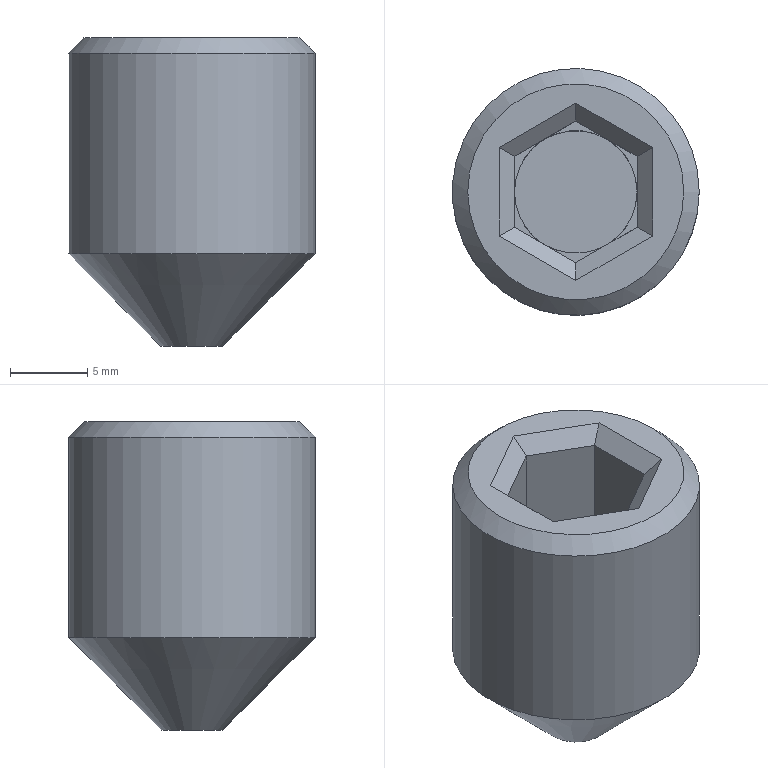Part | NX | features solid 2 | 1 solid | 25 faces | box 16 x 16 x 20 mm | volume 2801 mm3 | plane 21 | cylinder 2 | cone 2 | commonest cylinder face diameters 7.951 x1 16 x1
STEP:
#1=CARTESIAN_POINT('',(-112.,-5.,-5.));
#2=VERTEX_POINT('',#1);
#3=CARTESIAN_POINT('',(-120.,-5.,-5.));
#4=DIRECTION('',(0.,0.,1.));
#5=DIRECTION('',(1.,0.,0.));
#6=AXIS2_PLACEMENT_3D('',#3,#4,#5);
#7=CIRCLE('',#6,8.);
#8=EDGE_CURVE('',#2,#2,#7,.F.);
#9=ORIENTED_EDGE('',*,*,#8,.T.);
#10=EDGE_LOOP('',(#9));
#11=FACE_BOUND('',#10,.T.);
#12=CARTESIAN_POINT('',(-112.,-5.,-18.));
#13=VERTEX_POINT('',#12);
#14=CARTESIAN_POINT('',(-120.,-5.,-18.));
#15=DIRECTION('',(0.,0.,1.));
#16=DIRECTION('',(1.,0.,0.));
#17=AXIS2_PLACEMENT_3D('',#14,#15,#16);
#18=CIRCLE('',#17,8.);
#19=EDGE_CURVE('',#13,#13,#18,.F.);
#20=ORIENTED_EDGE('',*,*,#19,.F.);
#21=EDGE_LOOP('',(#20));
#22=FACE_BOUND('',#21,.T.);
#23=CARTESIAN_POINT('',(-120.,-5.,36.));
#24=DIRECTION('',(0.,0.,-1.));
#25=DIRECTION('',(-1.,0.,0.));
#26=AXIS2_PLACEMENT_3D('',#23,#24,#25);
#27=CYLINDRICAL_SURFACE('',#26,8.);
#28=ADVANCED_FACE('',(#11,#22),#27,.T.);
#29=CARTESIAN_POINT('',(-123.976,-5.,-11.));
#30=VERTEX_POINT('',#29);
#31=CARTESIAN_POINT('',(-121.988,-8.443,-11.));
#32=VERTEX_POINT('',#31);
#33=CARTESIAN_POINT('',(-120.,-5.,-11.));
#34=DIRECTION('',(0.,0.,-1.));
#35=DIRECTION('',(-1.,0.,0.));
#36=AXIS2_PLACEMENT_3D('',#33,#34,#35);
#37=CIRCLE('',#36,3.976);
#38=EDGE_CURVE('',#30,#32,#37,.F.);
#39=ORIENTED_EDGE('',*,*,#38,.F.);
#40=CARTESIAN_POINT('',(-123.976,-7.295,-11.));
#41=VERTEX_POINT('',#40);
#42=CARTESIAN_POINT('',(-123.976,-8.45,-11.));
#43=DIRECTION('',(0.,1.,0.));
#44=VECTOR('',#43,1000.);
#45=LINE('',#42,#44);
#46=EDGE_CURVE('',#41,#30,#45,.T.);
#47=ORIENTED_EDGE('',*,*,#46,.F.);
#48=CARTESIAN_POINT('',(-116.012,-11.893,-11.));
#49=DIRECTION('',(-0.866,0.5,0.));
#50=VECTOR('',#49,1000.);
#51=LINE('',#48,#50);
#52=EDGE_CURVE('',#32,#41,#51,.T.);
#53=ORIENTED_EDGE('',*,*,#52,.F.);
#54=EDGE_LOOP('',(#39,#47,#53));
#55=FACE_BOUND('',#54,.T.);
#56=CARTESIAN_POINT('',(-114.024,-8.45,-11.));
#57=DIRECTION('',(0.,0.,-1.));
#58=DIRECTION('',(-1.,0.,0.));
#59=AXIS2_PLACEMENT_3D('',#56,#57,#58);
#60=PLANE('',#59);
#61=ADVANCED_FACE('',(#55),#60,.F.);
#62=CARTESIAN_POINT('',(-118.012,-8.443,-11.));
#63=VERTEX_POINT('',#62);
#64=CARTESIAN_POINT('',(-120.,-5.,-11.));
#65=DIRECTION('',(0.,0.,-1.));
#66=DIRECTION('',(-1.,0.,0.));
#67=AXIS2_PLACEMENT_3D('',#64,#65,#66);
#68=CIRCLE('',#67,3.976);
#69=EDGE_CURVE('',#32,#63,#68,.F.);
#70=ORIENTED_EDGE('',*,*,#69,.F.);
#71=CARTESIAN_POINT('',(-120.,-9.591,-11.));
#72=VERTEX_POINT('',#71);
#73=CARTESIAN_POINT('',(-116.012,-11.893,-11.));
#74=DIRECTION('',(-0.866,0.5,0.));
#75=VECTOR('',#74,1000.);
#76=LINE('',#73,#75);
#77=EDGE_CURVE('',#72,#32,#76,.T.);
#78=ORIENTED_EDGE('',*,*,#77,.F.);
#79=CARTESIAN_POINT('',(-115.024,-6.718,-11.));
#80=DIRECTION('',(-0.866,-0.5,0.));
#81=VECTOR('',#80,1000.);
#82=LINE('',#79,#81);
#83=EDGE_CURVE('',#63,#72,#82,.T.);
#84=ORIENTED_EDGE('',*,*,#83,.F.);
#85=EDGE_LOOP('',(#70,#78,#84));
#86=FACE_BOUND('',#85,.T.);
#87=CARTESIAN_POINT('',(-114.024,-8.45,-11.));
#88=DIRECTION('',(0.,0.,-1.));
#89=DIRECTION('',(-1.,0.,0.));
#90=AXIS2_PLACEMENT_3D('',#87,#88,#89);
#91=PLANE('',#90);
#92=ADVANCED_FACE('',(#86),#91,.F.);
#93=CARTESIAN_POINT('',(-116.024,-5.,-11.));
#94=VERTEX_POINT('',#93);
#95=CARTESIAN_POINT('',(-120.,-5.,-11.));
#96=DIRECTION('',(0.,0.,-1.));
#97=DIRECTION('',(-1.,0.,0.));
#98=AXIS2_PLACEMENT_3D('',#95,#96,#97);
#99=CIRCLE('',#98,3.976);
#100=EDGE_CURVE('',#63,#94,#99,.F.);
#101=ORIENTED_EDGE('',*,*,#100,.F.);
#102=CARTESIAN_POINT('',(-116.024,-7.295,-11.));
#103=VERTEX_POINT('',#102);
#104=CARTESIAN_POINT('',(-115.024,-6.718,-11.));
#105=DIRECTION('',(-0.866,-0.5,0.));
#106=VECTOR('',#105,1000.);
#107=LINE('',#104,#106);
#108=EDGE_CURVE('',#103,#63,#107,.T.);
#109=ORIENTED_EDGE('',*,*,#108,.F.);
#110=CARTESIAN_POINT('',(-116.024,-8.45,-11.));
#111=DIRECTION('',(0.,-1.,0.));
#112=VECTOR('',#111,1000.);
#113=LINE('',#110,#112);
#114=EDGE_CURVE('',#94,#103,#113,.T.);
#115=ORIENTED_EDGE('',*,*,#114,.F.);
#116=EDGE_LOOP('',(#101,#109,#115));
#117=FACE_BOUND('',#116,.T.);
#118=CARTESIAN_POINT('',(-114.024,-8.45,-11.));
#119=DIRECTION('',(0.,0.,-1.));
#120=DIRECTION('',(-1.,0.,0.));
#121=AXIS2_PLACEMENT_3D('',#118,#119,#120);
#122=PLANE('',#121);
#123=ADVANCED_FACE('',(#117),#122,.F.);
#124=CARTESIAN_POINT('',(-118.012,-1.557,-11.));
#125=VERTEX_POINT('',#124);
#126=CARTESIAN_POINT('',(-120.,-5.,-11.));
#127=DIRECTION('',(0.,0.,-1.));
#128=DIRECTION('',(-1.,0.,0.));
#129=AXIS2_PLACEMENT_3D('',#126,#127,#128);
#130=CIRCLE('',#129,3.976);
#131=EDGE_CURVE('',#94,#125,#130,.F.);
#132=ORIENTED_EDGE('',*,*,#131,.F.);
#133=CARTESIAN_POINT('',(-116.024,-2.705,-11.));
#134=VERTEX_POINT('',#133);
#135=CARTESIAN_POINT('',(-116.024,-8.45,-11.));
#136=DIRECTION('',(0.,-1.,0.));
#137=VECTOR('',#136,1000.);
#138=LINE('',#135,#137);
#139=EDGE_CURVE('',#134,#94,#138,.T.);
#140=ORIENTED_EDGE('',*,*,#139,.F.);
#141=CARTESIAN_POINT('',(-112.037,-5.007,-11.));
#142=DIRECTION('',(0.866,-0.5,0.));
#143=VECTOR('',#142,1000.);
#144=LINE('',#141,#143);
#145=EDGE_CURVE('',#125,#134,#144,.T.);
#146=ORIENTED_EDGE('',*,*,#145,.F.);
#147=EDGE_LOOP('',(#132,#140,#146));
#148=FACE_BOUND('',#147,.T.);
#149=CARTESIAN_POINT('',(-114.024,-8.45,-11.));
#150=DIRECTION('',(0.,0.,-1.));
#151=DIRECTION('',(-1.,0.,0.));
#152=AXIS2_PLACEMENT_3D('',#149,#150,#151);
#153=PLANE('',#152);
#154=ADVANCED_FACE('',(#148),#153,.F.);
#155=CARTESIAN_POINT('',(-121.988,-1.557,-11.));
#156=VERTEX_POINT('',#155);
#157=CARTESIAN_POINT('',(-120.,-5.,-11.));
#158=DIRECTION('',(0.,0.,-1.));
#159=DIRECTION('',(-1.,0.,0.));
#160=AXIS2_PLACEMENT_3D('',#157,#158,#159);
#161=CIRCLE('',#160,3.976);
#162=EDGE_CURVE('',#125,#156,#161,.F.);
#163=ORIENTED_EDGE('',*,*,#162,.F.);
#164=CARTESIAN_POINT('',(-120.,-0.4094,-11.));
#165=VERTEX_POINT('',#164);
#166=CARTESIAN_POINT('',(-112.037,-5.007,-11.));
#167=DIRECTION('',(0.866,-0.5,0.));
#168=VECTOR('',#167,1000.);
#169=LINE('',#166,#168);
#170=EDGE_CURVE('',#165,#125,#169,.T.);
#171=ORIENTED_EDGE('',*,*,#170,.F.);
#172=CARTESIAN_POINT('',(-119.,0.1679,-11.));
#173=DIRECTION('',(0.866,0.5,0.));
#174=VECTOR('',#173,1000.);
#175=LINE('',#172,#174);
#176=EDGE_CURVE('',#156,#165,#175,.T.);
#177=ORIENTED_EDGE('',*,*,#176,.F.);
#178=EDGE_LOOP('',(#163,#171,#177));
#179=FACE_BOUND('',#178,.T.);
#180=CARTESIAN_POINT('',(-114.024,-8.45,-11.));
#181=DIRECTION('',(0.,0.,-1.));
#182=DIRECTION('',(-1.,0.,0.));
#183=AXIS2_PLACEMENT_3D('',#180,#181,#182);
#184=PLANE('',#183);
#185=ADVANCED_FACE('',(#179),#184,.F.);
#186=CARTESIAN_POINT('',(-120.,-5.,-11.));
#187=DIRECTION('',(0.,0.,-1.));
#188=DIRECTION('',(-1.,0.,0.));
#189=AXIS2_PLACEMENT_3D('',#186,#187,#188);
#190=CIRCLE('',#189,3.976);
#191=EDGE_CURVE('',#156,#30,#190,.F.);
#192=ORIENTED_EDGE('',*,*,#191,.F.);
#193=CARTESIAN_POINT('',(-123.976,-2.705,-11.));
#194=VERTEX_POINT('',#193);
#195=CARTESIAN_POINT('',(-119.,0.1679,-11.));
#196=DIRECTION('',(0.866,0.5,0.));
#197=VECTOR('',#196,1000.);
#198=LINE('',#195,#197);
#199=EDGE_CURVE('',#194,#156,#198,.T.);
#200=ORIENTED_EDGE('',*,*,#199,.F.);
#201=CARTESIAN_POINT('',(-123.976,-8.45,-11.));
#202=DIRECTION('',(0.,1.,0.));
#203=VECTOR('',#202,1000.);
#204=LINE('',#201,#203);
#205=EDGE_CURVE('',#30,#194,#204,.T.);
#206=ORIENTED_EDGE('',*,*,#205,.F.);
#207=EDGE_LOOP('',(#192,#200,#206));
#208=FACE_BOUND('',#207,.T.);
#209=CARTESIAN_POINT('',(-114.024,-8.45,-11.));
#210=DIRECTION('',(0.,0.,-1.));
#211=DIRECTION('',(-1.,0.,0.));
#212=AXIS2_PLACEMENT_3D('',#209,#210,#211);
#213=PLANE('',#212);
#214=ADVANCED_FACE('',(#208),#213,.F.);
#215=CARTESIAN_POINT('',(-113.,-5.,-4.));
#216=VERTEX_POINT('',#215);
#217=CARTESIAN_POINT('',(-120.,-5.,-4.));
#218=DIRECTION('',(0.,0.,1.));
#219=DIRECTION('',(1.,0.,0.));
#220=AXIS2_PLACEMENT_3D('',#217,#218,#219);
#221=CIRCLE('',#220,7.);
#222=EDGE_CURVE('',#216,#216,#221,.T.);
#223=ORIENTED_EDGE('',*,*,#222,.T.);
#224=EDGE_LOOP('',(#223));
#225=FACE_BOUND('',#224,.T.);
#226=CARTESIAN_POINT('',(-120.,0.7453,-4.));
#227=VERTEX_POINT('',#226);
#228=CARTESIAN_POINT('',(-115.024,-2.127,-4.));
#229=VERTEX_POINT('',#228);
#230=CARTESIAN_POINT('',(-115.524,-1.839,-4.));
#231=DIRECTION('',(0.866,-0.5,0.));
#232=VECTOR('',#231,1000.);
#233=LINE('',#230,#232);
#234=EDGE_CURVE('',#227,#229,#233,.T.);
#235=ORIENTED_EDGE('',*,*,#234,.T.);
#236=CARTESIAN_POINT('',(-115.024,-7.873,-4.));
#237=VERTEX_POINT('',#236);
#238=CARTESIAN_POINT('',(-115.024,-8.45,-4.));
#239=DIRECTION('',(0.,-1.,0.));
#240=VECTOR('',#239,1000.);
#241=LINE('',#238,#240);
#242=EDGE_CURVE('',#229,#237,#241,.T.);
#243=ORIENTED_EDGE('',*,*,#242,.T.);
#244=CARTESIAN_POINT('',(-120.,-10.745,-4.));
#245=VERTEX_POINT('',#244);
#246=CARTESIAN_POINT('',(-120.5,-11.034,-4.));
#247=DIRECTION('',(-0.866,-0.5,0.));
#248=VECTOR('',#247,1000.);
#249=LINE('',#246,#248);
#250=EDGE_CURVE('',#237,#245,#249,.T.);
#251=ORIENTED_EDGE('',*,*,#250,.T.);
#252=CARTESIAN_POINT('',(-124.976,-7.873,-4.));
#253=VERTEX_POINT('',#252);
#254=CARTESIAN_POINT('',(-125.476,-7.584,-4.));
#255=DIRECTION('',(-0.866,0.5,0.));
#256=VECTOR('',#255,1000.);
#257=LINE('',#254,#256);
#258=EDGE_CURVE('',#245,#253,#257,.T.);
#259=ORIENTED_EDGE('',*,*,#258,.T.);
#260=CARTESIAN_POINT('',(-124.976,-2.127,-4.));
#261=VERTEX_POINT('',#260);
#262=CARTESIAN_POINT('',(-124.976,-2.705,-4.));
#263=DIRECTION('',(0.,1.,0.));
#264=VECTOR('',#263,1000.);
#265=LINE('',#262,#264);
#266=EDGE_CURVE('',#253,#261,#265,.T.);
#267=ORIENTED_EDGE('',*,*,#266,.T.);
#268=CARTESIAN_POINT('',(-120.5,0.4566,-4.));
#269=DIRECTION('',(0.866,0.5,0.));
#270=VECTOR('',#269,1000.);
#271=LINE('',#268,#270);
#272=EDGE_CURVE('',#261,#227,#271,.T.);
#273=ORIENTED_EDGE('',*,*,#272,.T.);
#274=EDGE_LOOP('',(#235,#243,#251,#259,#267,#273));
#275=FACE_BOUND('',#274,.T.);
#276=CARTESIAN_POINT('',(-120.,-5.,-4.));
#277=DIRECTION('',(0.,0.,1.));
#278=DIRECTION('',(1.,0.,0.));
#279=AXIS2_PLACEMENT_3D('',#276,#277,#278);
#280=PLANE('',#279);
#281=ADVANCED_FACE('',(#225,#275),#280,.T.);
#282=CARTESIAN_POINT('',(-116.024,-7.295,-5.));
#283=VERTEX_POINT('',#282);
#284=CARTESIAN_POINT('',(-116.024,-7.295,36.));
#285=DIRECTION('',(0.,0.,-1.));
#286=VECTOR('',#285,1000.);
#287=LINE('',#284,#286);
#288=EDGE_CURVE('',#283,#103,#287,.T.);
#289=ORIENTED_EDGE('',*,*,#288,.F.);
#290=CARTESIAN_POINT('',(-116.024,-2.705,-5.));
#291=VERTEX_POINT('',#290);
#292=CARTESIAN_POINT('',(-116.024,-1.55,-5.));
#293=DIRECTION('',(0.,1.,0.));
#294=VECTOR('',#293,1000.);
#295=LINE('',#292,#294);
#296=EDGE_CURVE('',#283,#291,#295,.T.);
#297=ORIENTED_EDGE('',*,*,#296,.T.);
#298=CARTESIAN_POINT('',(-116.024,-2.705,36.));
#299=DIRECTION('',(0.,0.,-1.));
#300=VECTOR('',#299,1000.);
#301=LINE('',#298,#300);
#302=EDGE_CURVE('',#291,#134,#301,.T.);
#303=ORIENTED_EDGE('',*,*,#302,.T.);
#304=ORIENTED_EDGE('',*,*,#139,.T.);
#305=ORIENTED_EDGE('',*,*,#114,.T.);
#306=EDGE_LOOP('',(#289,#297,#303,#304,#305));
#307=FACE_BOUND('',#306,.T.);
#308=CARTESIAN_POINT('',(-116.024,-1.55,36.));
#309=DIRECTION('',(1.,0.,0.));
#310=DIRECTION('',(0.,0.,-1.));
#311=AXIS2_PLACEMENT_3D('',#308,#309,#310);
#312=PLANE('',#311);
#313=ADVANCED_FACE('',(#307),#312,.F.);
#314=CARTESIAN_POINT('',(-120.,-9.591,-5.));
#315=VERTEX_POINT('',#314);
#316=CARTESIAN_POINT('',(-120.,-9.591,36.));
#317=DIRECTION('',(0.,0.,-1.));
#318=VECTOR('',#317,1000.);
#319=LINE('',#316,#318);
#320=EDGE_CURVE('',#315,#72,#319,.T.);
#321=ORIENTED_EDGE('',*,*,#320,.F.);
#322=CARTESIAN_POINT('',(-116.024,-7.295,-5.));
#323=DIRECTION('',(0.866,0.5,0.));
#324=VECTOR('',#323,1000.);
#325=LINE('',#322,#324);
#326=EDGE_CURVE('',#315,#283,#325,.T.);
#327=ORIENTED_EDGE('',*,*,#326,.T.);
#328=ORIENTED_EDGE('',*,*,#288,.T.);
#329=ORIENTED_EDGE('',*,*,#108,.T.);
#330=ORIENTED_EDGE('',*,*,#83,.T.);
#331=EDGE_LOOP('',(#321,#327,#328,#329,#330));
#332=FACE_BOUND('',#331,.T.);
#333=CARTESIAN_POINT('',(-115.024,-6.718,36.));
#334=DIRECTION('',(0.5,-0.866,0.));
#335=DIRECTION('',(0.866,0.5,0.));
#336=AXIS2_PLACEMENT_3D('',#333,#334,#335);
#337=PLANE('',#336);
#338=ADVANCED_FACE('',(#332),#337,.F.);
#339=CARTESIAN_POINT('',(-123.976,-7.295,-5.));
#340=VERTEX_POINT('',#339);
#341=CARTESIAN_POINT('',(-123.976,-7.295,36.));
#342=DIRECTION('',(0.,0.,-1.));
#343=VECTOR('',#342,1000.);
#344=LINE('',#341,#343);
#345=EDGE_CURVE('',#340,#41,#344,.T.);
#346=ORIENTED_EDGE('',*,*,#345,.F.);
#347=CARTESIAN_POINT('',(-120.,-9.591,-5.));
#348=DIRECTION('',(0.866,-0.5,0.));
#349=VECTOR('',#348,1000.);
#350=LINE('',#347,#349);
#351=EDGE_CURVE('',#340,#315,#350,.T.);
#352=ORIENTED_EDGE('',*,*,#351,.T.);
#353=ORIENTED_EDGE('',*,*,#320,.T.);
#354=ORIENTED_EDGE('',*,*,#77,.T.);
#355=ORIENTED_EDGE('',*,*,#52,.T.);
#356=EDGE_LOOP('',(#346,#352,#353,#354,#355));
#357=FACE_BOUND('',#356,.T.);
#358=CARTESIAN_POINT('',(-119.,-10.168,36.));
#359=DIRECTION('',(-0.5,-0.866,0.));
#360=DIRECTION('',(0.866,-0.5,0.));
#361=AXIS2_PLACEMENT_3D('',#358,#359,#360);
#362=PLANE('',#361);
#363=ADVANCED_FACE('',(#357),#362,.F.);
#364=CARTESIAN_POINT('',(-123.976,-2.705,-5.));
#365=VERTEX_POINT('',#364);
#366=CARTESIAN_POINT('',(-123.976,-2.705,36.));
#367=DIRECTION('',(0.,0.,-1.));
#368=VECTOR('',#367,1000.);
#369=LINE('',#366,#368);
#370=EDGE_CURVE('',#365,#194,#369,.T.);
#371=ORIENTED_EDGE('',*,*,#370,.F.);
#372=CARTESIAN_POINT('',(-123.976,-7.295,-5.));
#373=DIRECTION('',(0.,-1.,0.));
#374=VECTOR('',#373,1000.);
#375=LINE('',#372,#374);
#376=EDGE_CURVE('',#365,#340,#375,.T.);
#377=ORIENTED_EDGE('',*,*,#376,.T.);
#378=ORIENTED_EDGE('',*,*,#345,.T.);
#379=ORIENTED_EDGE('',*,*,#46,.T.);
#380=ORIENTED_EDGE('',*,*,#205,.T.);
#381=EDGE_LOOP('',(#371,#377,#378,#379,#380));
#382=FACE_BOUND('',#381,.T.);
#383=CARTESIAN_POINT('',(-123.976,-8.45,36.));
#384=DIRECTION('',(-1.,0.,0.));
#385=DIRECTION('',(0.,0.,1.));
#386=AXIS2_PLACEMENT_3D('',#383,#384,#385);
#387=PLANE('',#386);
#388=ADVANCED_FACE('',(#382),#387,.F.);
#389=CARTESIAN_POINT('',(-120.,-0.4094,-5.));
#390=VERTEX_POINT('',#389);
#391=CARTESIAN_POINT('',(-120.,-0.4094,36.));
#392=DIRECTION('',(0.,0.,-1.));
#393=VECTOR('',#392,1000.);
#394=LINE('',#391,#393);
#395=EDGE_CURVE('',#390,#165,#394,.T.);
#396=ORIENTED_EDGE('',*,*,#395,.F.);
#397=CARTESIAN_POINT('',(-124.976,-3.282,-5.));
#398=DIRECTION('',(-0.866,-0.5,0.));
#399=VECTOR('',#398,1000.);
#400=LINE('',#397,#399);
#401=EDGE_CURVE('',#390,#365,#400,.T.);
#402=ORIENTED_EDGE('',*,*,#401,.T.);
#403=ORIENTED_EDGE('',*,*,#370,.T.);
#404=ORIENTED_EDGE('',*,*,#199,.T.);
#405=ORIENTED_EDGE('',*,*,#176,.T.);
#406=EDGE_LOOP('',(#396,#402,#403,#404,#405));
#407=FACE_BOUND('',#406,.T.);
#408=CARTESIAN_POINT('',(-124.976,-3.282,36.));
#409=DIRECTION('',(-0.5,0.866,0.));
#410=DIRECTION('',(-0.866,-0.5,0.));
#411=AXIS2_PLACEMENT_3D('',#408,#409,#410);
#412=PLANE('',#411);
#413=ADVANCED_FACE('',(#407),#412,.F.);
#414=ORIENTED_EDGE('',*,*,#302,.F.);
#415=CARTESIAN_POINT('',(-121.,0.1679,-5.));
#416=DIRECTION('',(-0.866,0.5,0.));
#417=VECTOR('',#416,1000.);
#418=LINE('',#415,#417);
#419=EDGE_CURVE('',#291,#390,#418,.T.);
#420=ORIENTED_EDGE('',*,*,#419,.T.);
#421=ORIENTED_EDGE('',*,*,#395,.T.);
#422=ORIENTED_EDGE('',*,*,#170,.T.);
#423=ORIENTED_EDGE('',*,*,#145,.T.);
#424=EDGE_LOOP('',(#414,#420,#421,#422,#423));
#425=FACE_BOUND('',#424,.T.);
#426=CARTESIAN_POINT('',(-121.,0.1679,36.));
#427=DIRECTION('',(0.5,0.866,0.));
#428=DIRECTION('',(-0.866,0.5,0.));
#429=AXIS2_PLACEMENT_3D('',#426,#427,#428);
#430=PLANE('',#429);
#431=ADVANCED_FACE('',(#425),#430,.F.);
#432=ORIENTED_EDGE('',*,*,#131,.T.);
#433=ORIENTED_EDGE('',*,*,#162,.T.);
#434=ORIENTED_EDGE('',*,*,#191,.T.);
#435=ORIENTED_EDGE('',*,*,#38,.T.);
#436=ORIENTED_EDGE('',*,*,#69,.T.);
#437=ORIENTED_EDGE('',*,*,#100,.T.);
#438=EDGE_LOOP('',(#432,#433,#434,#435,#436,#437));
#439=FACE_BOUND('',#438,.T.);
#440=CARTESIAN_POINT('',(-116.024,-5.,-13.4));
#441=VERTEX_POINT('',#440);
#442=CARTESIAN_POINT('',(-120.,-5.,-13.4));
#443=DIRECTION('',(0.,0.,1.));
#444=DIRECTION('',(1.,0.,0.));
#445=AXIS2_PLACEMENT_3D('',#442,#443,#444);
#446=CIRCLE('',#445,3.976);
#447=EDGE_CURVE('',#441,#441,#446,.T.);
#448=ORIENTED_EDGE('',*,*,#447,.F.);
#449=EDGE_LOOP('',(#448));
#450=FACE_BOUND('',#449,.T.);
#451=CARTESIAN_POINT('',(-120.,-5.,-11.));
#452=DIRECTION('',(0.,0.,-1.));
#453=DIRECTION('',(-1.,0.,0.));
#454=AXIS2_PLACEMENT_3D('',#451,#452,#453);
#455=CYLINDRICAL_SURFACE('',#454,3.976);
#456=ADVANCED_FACE('',(#439,#450),#455,.F.);
#457=ORIENTED_EDGE('',*,*,#447,.T.);
#458=EDGE_LOOP('',(#457));
#459=FACE_BOUND('',#458,.T.);
#460=CARTESIAN_POINT('',(-120.,-5.,-13.4));
#461=DIRECTION('',(0.,0.,1.));
#462=DIRECTION('',(1.,0.,0.));
#463=AXIS2_PLACEMENT_3D('',#460,#461,#462);
#464=PLANE('',#463);
#465=ADVANCED_FACE('',(#459),#464,.T.);
#466=CARTESIAN_POINT('',(-118.,-5.,-24.));
#467=VERTEX_POINT('',#466);
#468=CARTESIAN_POINT('',(-120.,-5.,-24.));
#469=DIRECTION('',(0.,0.,1.));
#470=DIRECTION('',(1.,0.,0.));
#471=AXIS2_PLACEMENT_3D('',#468,#469,#470);
#472=CIRCLE('',#471,2.);
#473=EDGE_CURVE('',#467,#467,#472,.T.);
#474=ORIENTED_EDGE('',*,*,#473,.T.);
#475=EDGE_LOOP('',(#474));
#476=FACE_BOUND('',#475,.T.);
#477=ORIENTED_EDGE('',*,*,#19,.T.);
#478=EDGE_LOOP('',(#477));
#479=FACE_BOUND('',#478,.T.);
#480=CARTESIAN_POINT('',(-120.,-5.,-23.));
#481=DIRECTION('',(0.,0.,1.));
#482=DIRECTION('',(-1.,0.,0.));
#483=AXIS2_PLACEMENT_3D('',#480,#481,#482);
#484=CONICAL_SURFACE('',#483,3.,0.7854);
#485=ADVANCED_FACE('',(#476,#479),#484,.T.);
#486=ORIENTED_EDGE('',*,*,#473,.F.);
#487=EDGE_LOOP('',(#486));
#488=FACE_BOUND('',#487,.T.);
#489=CARTESIAN_POINT('',(-120.,-5.,-24.));
#490=DIRECTION('',(0.,0.,1.));
#491=DIRECTION('',(1.,0.,0.));
#492=AXIS2_PLACEMENT_3D('',#489,#490,#491);
#493=PLANE('',#492);
#494=ADVANCED_FACE('',(#488),#493,.F.);
#495=ORIENTED_EDGE('',*,*,#376,.F.);
#496=CARTESIAN_POINT('',(-124.265,-2.538,-4.711));
#497=DIRECTION('',(-0.6547,0.378,0.6547));
#498=VECTOR('',#497,1000.);
#499=LINE('',#496,#498);
#500=EDGE_CURVE('',#365,#261,#499,.T.);
#501=ORIENTED_EDGE('',*,*,#500,.T.);
#502=ORIENTED_EDGE('',*,*,#266,.F.);
#503=CARTESIAN_POINT('',(-122.554,-6.475,-6.422));
#504=DIRECTION('',(0.6547,0.378,-0.6547));
#505=VECTOR('',#504,1000.);
#506=LINE('',#503,#505);
#507=EDGE_CURVE('',#253,#340,#506,.T.);
#508=ORIENTED_EDGE('',*,*,#507,.T.);
#509=EDGE_LOOP('',(#495,#501,#502,#508));
#510=FACE_BOUND('',#509,.T.);
#511=CARTESIAN_POINT('',(-123.976,-8.45,-5.));
#512=DIRECTION('',(0.7071,0.,0.7071));
#513=DIRECTION('',(0.7071,0.,-0.7071));
#514=AXIS2_PLACEMENT_3D('',#511,#512,#513);
#515=PLANE('',#514);
#516=ADVANCED_FACE('',(#510),#515,.T.);
#517=ORIENTED_EDGE('',*,*,#500,.F.);
#518=ORIENTED_EDGE('',*,*,#401,.F.);
#519=CARTESIAN_POINT('',(-120.,-0.07949,-4.714));
#520=DIRECTION('',(0.,0.7559,0.6547));
#521=VECTOR('',#520,1000.);
#522=LINE('',#519,#521);
#523=EDGE_CURVE('',#390,#227,#522,.T.);
#524=ORIENTED_EDGE('',*,*,#523,.T.);
#525=ORIENTED_EDGE('',*,*,#272,.F.);
#526=EDGE_LOOP('',(#517,#518,#524,#525));
#527=FACE_BOUND('',#526,.T.);
#528=CARTESIAN_POINT('',(-122.488,-0.691,-4.));
#529=DIRECTION('',(0.3536,-0.6124,0.7071));
#530=DIRECTION('',(0.,-0.7559,-0.6547));
#531=AXIS2_PLACEMENT_3D('',#528,#529,#530);
#532=PLANE('',#531);
#533=ADVANCED_FACE('',(#527),#532,.T.);
#534=ORIENTED_EDGE('',*,*,#419,.F.);
#535=CARTESIAN_POINT('',(-115.739,-2.54,-4.714));
#536=DIRECTION('',(0.6547,0.378,0.6547));
#537=VECTOR('',#536,1000.);
#538=LINE('',#535,#537);
#539=EDGE_CURVE('',#291,#229,#538,.T.);
#540=ORIENTED_EDGE('',*,*,#539,.T.);
#541=ORIENTED_EDGE('',*,*,#234,.F.);
#542=ORIENTED_EDGE('',*,*,#523,.F.);
#543=EDGE_LOOP('',(#534,#540,#541,#542));
#544=FACE_BOUND('',#543,.T.);
#545=CARTESIAN_POINT('',(-121.,0.1679,-5.));
#546=DIRECTION('',(-0.3536,-0.6124,0.7071));
#547=DIRECTION('',(0.,-0.7559,-0.6547));
#548=AXIS2_PLACEMENT_3D('',#545,#546,#547);
#549=PLANE('',#548);
#550=ADVANCED_FACE('',(#544),#549,.T.);
#551=ORIENTED_EDGE('',*,*,#507,.F.);
#552=ORIENTED_EDGE('',*,*,#258,.F.);
#553=CARTESIAN_POINT('',(-120.,-7.949,-6.422));
#554=DIRECTION('',(0.,0.7559,-0.6547));
#555=VECTOR('',#554,1000.);
#556=LINE('',#553,#555);
#557=EDGE_CURVE('',#245,#315,#556,.T.);
#558=ORIENTED_EDGE('',*,*,#557,.T.);
#559=ORIENTED_EDGE('',*,*,#351,.F.);
#560=EDGE_LOOP('',(#551,#552,#558,#559));
#561=FACE_BOUND('',#560,.T.);
#562=CARTESIAN_POINT('',(-119.,-10.168,-5.));
#563=DIRECTION('',(0.3536,0.6124,0.7071));
#564=DIRECTION('',(0.,-0.7559,0.6547));
#565=AXIS2_PLACEMENT_3D('',#562,#563,#564);
#566=PLANE('',#565);
#567=ADVANCED_FACE('',(#561),#566,.T.);
#568=ORIENTED_EDGE('',*,*,#557,.F.);
#569=ORIENTED_EDGE('',*,*,#250,.F.);
#570=CARTESIAN_POINT('',(-117.446,-6.475,-6.422));
#571=DIRECTION('',(-0.6547,0.378,-0.6547));
#572=VECTOR('',#571,1000.);
#573=LINE('',#570,#572);
#574=EDGE_CURVE('',#237,#283,#573,.T.);
#575=ORIENTED_EDGE('',*,*,#574,.T.);
#576=ORIENTED_EDGE('',*,*,#326,.F.);
#577=EDGE_LOOP('',(#568,#569,#575,#576));
#578=FACE_BOUND('',#577,.T.);
#579=CARTESIAN_POINT('',(-115.024,-6.718,-5.));
#580=DIRECTION('',(-0.3536,0.6124,0.7071));
#581=DIRECTION('',(0.,-0.7559,0.6547));
#582=AXIS2_PLACEMENT_3D('',#579,#580,#581);
#583=PLANE('',#582);
#584=ADVANCED_FACE('',(#578),#583,.T.);
#585=ORIENTED_EDGE('',*,*,#574,.F.);
#586=ORIENTED_EDGE('',*,*,#242,.F.);
#587=ORIENTED_EDGE('',*,*,#539,.F.);
#588=ORIENTED_EDGE('',*,*,#296,.F.);
#589=EDGE_LOOP('',(#585,#586,#587,#588));
#590=FACE_BOUND('',#589,.T.);
#591=CARTESIAN_POINT('',(-116.024,-1.55,-5.));
#592=DIRECTION('',(-0.7071,0.,0.7071));
#593=DIRECTION('',(0.7071,0.,0.7071));
#594=AXIS2_PLACEMENT_3D('',#591,#592,#593);
#595=PLANE('',#594);
#596=ADVANCED_FACE('',(#590),#595,.T.);
#597=ORIENTED_EDGE('',*,*,#8,.F.);
#598=EDGE_LOOP('',(#597));
#599=FACE_BOUND('',#598,.T.);
#600=ORIENTED_EDGE('',*,*,#222,.F.);
#601=EDGE_LOOP('',(#600));
#602=FACE_BOUND('',#601,.T.);
#603=CARTESIAN_POINT('',(-120.,-5.,-4.));
#604=DIRECTION('',(0.,0.,-1.));
#605=DIRECTION('',(-1.,0.,0.));
#606=AXIS2_PLACEMENT_3D('',#603,#604,#605);
#607=CONICAL_SURFACE('',#606,7.,0.7854);
#608=ADVANCED_FACE('',(#599,#602),#607,.T.);
#609=CLOSED_SHELL('',(#28,#61,#92,#123,#154,#185,#214,#281,#313,#338,#363,#388,#413,#431,#456,#465,#485,#494,#516,#533,#550,#567,#584,#596,#608));
#610=MANIFOLD_SOLID_BREP('',#609);
#611=(LENGTH_UNIT()NAMED_UNIT(*)SI_UNIT(.MILLI.,.METRE.));
#612=UNCERTAINTY_MEASURE_WITH_UNIT(LENGTH_MEASURE(0.00001),#611,'','');
#613=(NAMED_UNIT(*)PLANE_ANGLE_UNIT()SI_UNIT($,.RADIAN.));
#614=(NAMED_UNIT(*)SI_UNIT($,.STERADIAN.)SOLID_ANGLE_UNIT());
#615=(GEOMETRIC_REPRESENTATION_CONTEXT(3)GLOBAL_UNCERTAINTY_ASSIGNED_CONTEXT((#612))GLOBAL_UNIT_ASSIGNED_CONTEXT((#611,#613,#614))REPRESENTATION_CONTEXT('',''));
#616=ADVANCED_BREP_SHAPE_REPRESENTATION('',(#610),#615);